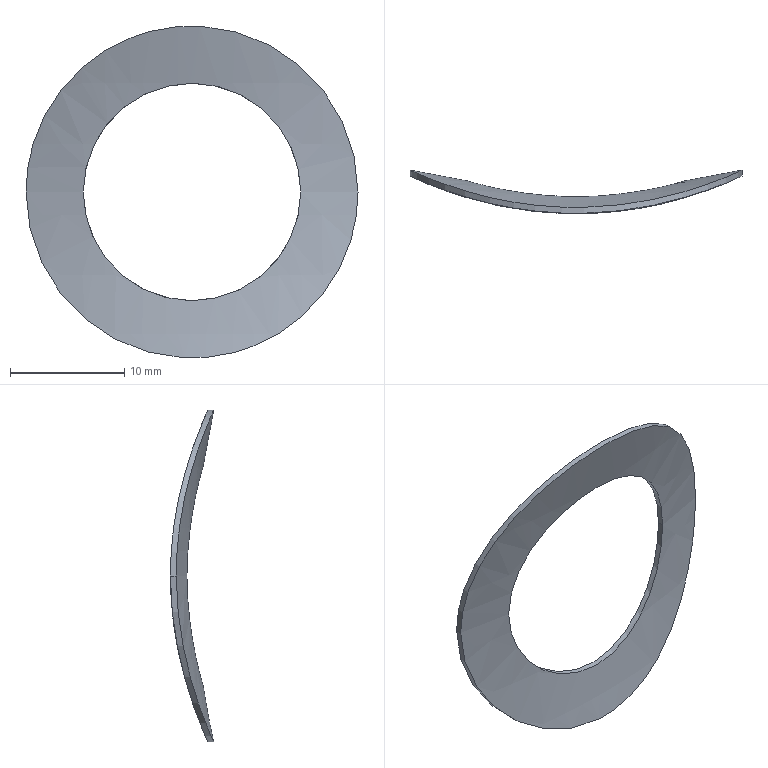Part | NX | features BREP 1 | 1 solid | 6 faces | box 29 x 3.789 x 29 mm | volume 191.933 mm3 | cylinder 4 | torus 2 | commonest cylinder face diameters 19 x2 29 x2
STEP:
#1=CARTESIAN_POINT('',(-264.193,-157.362,-153.339));
#2=VERTEX_POINT('',#1);
#3=CARTESIAN_POINT('',(-293.193,-157.362,-153.339));
#4=VERTEX_POINT('',#3);
#5=CARTESIAN_POINT('',(-264.193,-157.362,-153.339));
#6=CARTESIAN_POINT('',(-264.193,-157.362,-149.457));
#7=CARTESIAN_POINT('',(-266.594,-158.58,-143.888));
#8=CARTESIAN_POINT('',(-272.929,-160.276,-139.628));
#9=CARTESIAN_POINT('',(-278.667,-160.818,-138.448));
#10=CARTESIAN_POINT('',(-284.442,-160.279,-139.615));
#11=CARTESIAN_POINT('',(-289.203,-159.013,-142.828));
#12=CARTESIAN_POINT('',(-292.404,-157.737,-147.574));
#13=CARTESIAN_POINT('',(-293.193,-157.362,-151.397));
#14=CARTESIAN_POINT('',(-293.193,-157.362,-153.339));
#15=B_SPLINE_CURVE_WITH_KNOTS('',3,(#5,#6,#7,#8,#9,#10,#11,#12,#13,#14),.UNSPECIFIED.,.F.,.F.,(4,1,1,1,1,1,1,4),(0.,0.01147,0.0172,0.02294,0.02867,0.03441,0.04014,0.04588),.UNSPECIFIED.);
#16=EDGE_CURVE('',#2,#4,#15,.T.);
#17=ORIENTED_EDGE('',*,*,#16,.F.);
#18=CARTESIAN_POINT('',(-293.193,-157.362,-153.339));
#19=CARTESIAN_POINT('',(-293.193,-157.362,-157.221));
#20=CARTESIAN_POINT('',(-290.792,-158.58,-162.79));
#21=CARTESIAN_POINT('',(-284.457,-160.276,-167.05));
#22=CARTESIAN_POINT('',(-278.719,-160.818,-168.23));
#23=CARTESIAN_POINT('',(-272.944,-160.279,-167.063));
#24=CARTESIAN_POINT('',(-268.183,-159.013,-163.85));
#25=CARTESIAN_POINT('',(-264.982,-157.737,-159.104));
#26=CARTESIAN_POINT('',(-264.193,-157.362,-155.281));
#27=CARTESIAN_POINT('',(-264.193,-157.362,-153.339));
#28=B_SPLINE_CURVE_WITH_KNOTS('',3,(#18,#19,#20,#21,#22,#23,#24,#25,#26,#27),.UNSPECIFIED.,.F.,.F.,(4,1,1,1,1,1,1,4),(0.,0.01147,0.0172,0.02294,0.02867,0.03441,0.04014,0.04588),.UNSPECIFIED.);
#29=EDGE_CURVE('',#4,#2,#28,.T.);
#30=ORIENTED_EDGE('',*,*,#29,.F.);
#31=EDGE_LOOP('',(#17,#30));
#32=FACE_BOUND('',#31,.T.);
#33=CARTESIAN_POINT('',(-269.193,-158.302,-153.339));
#34=VERTEX_POINT('',#33);
#35=CARTESIAN_POINT('',(-288.193,-158.302,-153.339));
#36=VERTEX_POINT('',#35);
#37=CARTESIAN_POINT('',(-269.193,-158.302,-153.339));
#38=CARTESIAN_POINT('',(-269.193,-158.302,-150.815));
#39=CARTESIAN_POINT('',(-271.253,-159.004,-145.916));
#40=CARTESIAN_POINT('',(-278.678,-160.045,-142.802));
#41=CARTESIAN_POINT('',(-286.137,-159.005,-145.911));
#42=CARTESIAN_POINT('',(-288.193,-158.302,-150.815));
#43=CARTESIAN_POINT('',(-288.193,-158.302,-153.339));
#44=B_SPLINE_CURVE_WITH_KNOTS('',3,(#37,#38,#39,#40,#41,#42,#43),.UNSPECIFIED.,.F.,.F.,(4,1,1,1,4),(0.,0.007462,0.01492,0.02239,0.02985),.UNSPECIFIED.);
#45=EDGE_CURVE('',#34,#36,#44,.T.);
#46=ORIENTED_EDGE('',*,*,#45,.T.);
#47=CARTESIAN_POINT('',(-288.193,-158.302,-153.339));
#48=CARTESIAN_POINT('',(-288.193,-158.302,-155.863));
#49=CARTESIAN_POINT('',(-286.133,-159.004,-160.762));
#50=CARTESIAN_POINT('',(-278.708,-160.045,-163.876));
#51=CARTESIAN_POINT('',(-271.249,-159.005,-160.767));
#52=CARTESIAN_POINT('',(-269.193,-158.302,-155.863));
#53=CARTESIAN_POINT('',(-269.193,-158.302,-153.339));
#54=B_SPLINE_CURVE_WITH_KNOTS('',3,(#47,#48,#49,#50,#51,#52,#53),.UNSPECIFIED.,.F.,.F.,(4,1,1,1,4),(0.,0.007462,0.01492,0.02239,0.02985),.UNSPECIFIED.);
#55=EDGE_CURVE('',#36,#34,#54,.T.);
#56=ORIENTED_EDGE('',*,*,#55,.T.);
#57=EDGE_LOOP('',(#46,#56));
#58=FACE_BOUND('',#57,.T.);
#59=CARTESIAN_POINT('',(-278.693,-94.,-153.339));
#60=DIRECTION('',(0.,0.,1.));
#61=DIRECTION('',(0.2246,0.9745,0.));
#62=AXIS2_PLACEMENT_3D('',#59,#60,#61);
#63=TOROIDAL_SURFACE('',#62,130.,65.);
#64=ADVANCED_FACE('',(#32,#58),#63,.T.);
#65=CARTESIAN_POINT('',(-264.193,-157.875,-153.339));
#66=VERTEX_POINT('',#65);
#67=CARTESIAN_POINT('',(-264.193,-157.875,-153.339));
#68=DIRECTION('',(0.,1.,0.));
#69=VECTOR('',#68,1000.);
#70=LINE('',#67,#69);
#71=EDGE_CURVE('',#2,#66,#70,.F.);
#72=ORIENTED_EDGE('',*,*,#71,.F.);
#73=ORIENTED_EDGE('',*,*,#16,.T.);
#74=CARTESIAN_POINT('',(-293.193,-157.875,-153.339));
#75=VERTEX_POINT('',#74);
#76=CARTESIAN_POINT('',(-293.193,-157.875,-153.339));
#77=DIRECTION('',(0.,1.,0.));
#78=VECTOR('',#77,1000.);
#79=LINE('',#76,#78);
#80=EDGE_CURVE('',#4,#75,#79,.F.);
#81=ORIENTED_EDGE('',*,*,#80,.T.);
#82=CARTESIAN_POINT('',(-264.193,-157.875,-153.339));
#83=CARTESIAN_POINT('',(-264.193,-157.875,-149.457));
#84=CARTESIAN_POINT('',(-266.594,-159.092,-143.888));
#85=CARTESIAN_POINT('',(-272.929,-160.789,-139.628));
#86=CARTESIAN_POINT('',(-278.667,-161.331,-138.448));
#87=CARTESIAN_POINT('',(-284.442,-160.792,-139.615));
#88=CARTESIAN_POINT('',(-289.203,-159.525,-142.827));
#89=CARTESIAN_POINT('',(-292.404,-158.25,-147.574));
#90=CARTESIAN_POINT('',(-293.193,-157.875,-151.397));
#91=CARTESIAN_POINT('',(-293.193,-157.875,-153.339));
#92=B_SPLINE_CURVE_WITH_KNOTS('',3,(#82,#83,#84,#85,#86,#87,#88,#89,#90,#91),.UNSPECIFIED.,.F.,.F.,(4,1,1,1,1,1,1,4),(0.,0.01147,0.0172,0.02294,0.02867,0.03441,0.04014,0.04588),.UNSPECIFIED.);
#93=EDGE_CURVE('',#66,#75,#92,.T.);
#94=ORIENTED_EDGE('',*,*,#93,.F.);
#95=EDGE_LOOP('',(#72,#73,#81,#94));
#96=FACE_BOUND('',#95,.T.);
#97=CARTESIAN_POINT('',(-278.693,-157.319,-153.339));
#98=DIRECTION('',(0.,-1.,0.));
#99=DIRECTION('',(-1.,0.,0.));
#100=AXIS2_PLACEMENT_3D('',#97,#98,#99);
#101=CYLINDRICAL_SURFACE('',#100,14.5);
#102=ADVANCED_FACE('',(#96),#101,.T.);
#103=ORIENTED_EDGE('',*,*,#71,.T.);
#104=CARTESIAN_POINT('',(-293.193,-157.875,-153.339));
#105=CARTESIAN_POINT('',(-293.193,-157.875,-157.221));
#106=CARTESIAN_POINT('',(-290.792,-159.092,-162.79));
#107=CARTESIAN_POINT('',(-284.457,-160.789,-167.05));
#108=CARTESIAN_POINT('',(-278.719,-161.331,-168.23));
#109=CARTESIAN_POINT('',(-272.944,-160.792,-167.063));
#110=CARTESIAN_POINT('',(-268.183,-159.525,-163.851));
#111=CARTESIAN_POINT('',(-264.982,-158.25,-159.104));
#112=CARTESIAN_POINT('',(-264.193,-157.875,-155.281));
#113=CARTESIAN_POINT('',(-264.193,-157.875,-153.339));
#114=B_SPLINE_CURVE_WITH_KNOTS('',3,(#104,#105,#106,#107,#108,#109,#110,#111,#112,#113),.UNSPECIFIED.,.F.,.F.,(4,1,1,1,1,1,1,4),(0.,0.01147,0.0172,0.02294,0.02867,0.03441,0.04014,0.04588),.UNSPECIFIED.);
#115=EDGE_CURVE('',#75,#66,#114,.T.);
#116=ORIENTED_EDGE('',*,*,#115,.F.);
#117=ORIENTED_EDGE('',*,*,#80,.F.);
#118=ORIENTED_EDGE('',*,*,#29,.T.);
#119=EDGE_LOOP('',(#103,#116,#117,#118));
#120=FACE_BOUND('',#119,.T.);
#121=CARTESIAN_POINT('',(-278.693,-157.319,-153.339));
#122=DIRECTION('',(0.,-1.,0.));
#123=DIRECTION('',(-1.,0.,0.));
#124=AXIS2_PLACEMENT_3D('',#121,#122,#123);
#125=CYLINDRICAL_SURFACE('',#124,14.5);
#126=ADVANCED_FACE('',(#120),#125,.T.);
#127=CARTESIAN_POINT('',(-269.193,-158.807,-153.339));
#128=VERTEX_POINT('',#127);
#129=CARTESIAN_POINT('',(-269.193,-158.807,-153.339));
#130=DIRECTION('',(0.,1.,0.));
#131=VECTOR('',#130,1000.);
#132=LINE('',#129,#131);
#133=EDGE_CURVE('',#34,#128,#132,.F.);
#134=ORIENTED_EDGE('',*,*,#133,.F.);
#135=ORIENTED_EDGE('',*,*,#55,.F.);
#136=CARTESIAN_POINT('',(-288.193,-158.807,-153.339));
#137=VERTEX_POINT('',#136);
#138=CARTESIAN_POINT('',(-288.193,-158.807,-153.339));
#139=DIRECTION('',(0.,1.,0.));
#140=VECTOR('',#139,1000.);
#141=LINE('',#138,#140);
#142=EDGE_CURVE('',#36,#137,#141,.F.);
#143=ORIENTED_EDGE('',*,*,#142,.T.);
#144=CARTESIAN_POINT('',(-269.193,-158.807,-153.339));
#145=CARTESIAN_POINT('',(-269.193,-158.807,-155.863));
#146=CARTESIAN_POINT('',(-271.253,-159.509,-160.762));
#147=CARTESIAN_POINT('',(-278.678,-160.55,-163.876));
#148=CARTESIAN_POINT('',(-286.137,-159.51,-160.767));
#149=CARTESIAN_POINT('',(-288.193,-158.807,-155.863));
#150=CARTESIAN_POINT('',(-288.193,-158.807,-153.339));
#151=B_SPLINE_CURVE_WITH_KNOTS('',3,(#144,#145,#146,#147,#148,#149,#150),.UNSPECIFIED.,.F.,.F.,(4,1,1,1,4),(0.,0.007462,0.01492,0.02239,0.02985),.UNSPECIFIED.);
#152=EDGE_CURVE('',#128,#137,#151,.T.);
#153=ORIENTED_EDGE('',*,*,#152,.F.);
#154=EDGE_LOOP('',(#134,#135,#143,#153));
#155=FACE_BOUND('',#154,.T.);
#156=CARTESIAN_POINT('',(-278.693,-158.289,-153.339));
#157=DIRECTION('',(0.,-1.,0.));
#158=DIRECTION('',(-1.,0.,0.));
#159=AXIS2_PLACEMENT_3D('',#156,#157,#158);
#160=CYLINDRICAL_SURFACE('',#159,9.5);
#161=ADVANCED_FACE('',(#155),#160,.F.);
#162=ORIENTED_EDGE('',*,*,#133,.T.);
#163=CARTESIAN_POINT('',(-288.193,-158.807,-153.339));
#164=CARTESIAN_POINT('',(-288.193,-158.807,-150.815));
#165=CARTESIAN_POINT('',(-286.133,-159.509,-145.916));
#166=CARTESIAN_POINT('',(-278.708,-160.55,-142.802));
#167=CARTESIAN_POINT('',(-271.249,-159.51,-145.911));
#168=CARTESIAN_POINT('',(-269.193,-158.807,-150.815));
#169=CARTESIAN_POINT('',(-269.193,-158.807,-153.339));
#170=B_SPLINE_CURVE_WITH_KNOTS('',3,(#163,#164,#165,#166,#167,#168,#169),.UNSPECIFIED.,.F.,.F.,(4,1,1,1,4),(0.,0.007462,0.01492,0.02239,0.02985),.UNSPECIFIED.);
#171=EDGE_CURVE('',#137,#128,#170,.T.);
#172=ORIENTED_EDGE('',*,*,#171,.F.);
#173=ORIENTED_EDGE('',*,*,#142,.F.);
#174=ORIENTED_EDGE('',*,*,#45,.F.);
#175=EDGE_LOOP('',(#162,#172,#173,#174));
#176=FACE_BOUND('',#175,.T.);
#177=CARTESIAN_POINT('',(-278.693,-158.289,-153.339));
#178=DIRECTION('',(0.,-1.,0.));
#179=DIRECTION('',(-1.,0.,0.));
#180=AXIS2_PLACEMENT_3D('',#177,#178,#179);
#181=CYLINDRICAL_SURFACE('',#180,9.5);
#182=ADVANCED_FACE('',(#176),#181,.F.);
#183=ORIENTED_EDGE('',*,*,#115,.T.);
#184=ORIENTED_EDGE('',*,*,#93,.T.);
#185=EDGE_LOOP('',(#183,#184));
#186=FACE_BOUND('',#185,.T.);
#187=ORIENTED_EDGE('',*,*,#171,.T.);
#188=ORIENTED_EDGE('',*,*,#152,.T.);
#189=EDGE_LOOP('',(#187,#188));
#190=FACE_BOUND('',#189,.T.);
#191=CARTESIAN_POINT('',(-278.693,-94.,-153.339));
#192=DIRECTION('',(0.,0.,1.));
#193=DIRECTION('',(0.2229,0.9748,0.));
#194=AXIS2_PLACEMENT_3D('',#191,#192,#193);
#195=TOROIDAL_SURFACE('',#194,130.,64.5);
#196=ADVANCED_FACE('',(#186,#190),#195,.F.);
#197=CLOSED_SHELL('',(#64,#102,#126,#161,#182,#196));
#198=MANIFOLD_SOLID_BREP('',#197);
#199=(LENGTH_UNIT()NAMED_UNIT(*)SI_UNIT(.MILLI.,.METRE.));
#200=UNCERTAINTY_MEASURE_WITH_UNIT(LENGTH_MEASURE(0.0508),#199,'','');
#201=(NAMED_UNIT(*)PLANE_ANGLE_UNIT()SI_UNIT($,.RADIAN.));
#202=(NAMED_UNIT(*)SI_UNIT($,.STERADIAN.)SOLID_ANGLE_UNIT());
#203=(GEOMETRIC_REPRESENTATION_CONTEXT(3)GLOBAL_UNCERTAINTY_ASSIGNED_CONTEXT((#200))GLOBAL_UNIT_ASSIGNED_CONTEXT((#199,#201,#202))REPRESENTATION_CONTEXT('',''));
#204=ADVANCED_BREP_SHAPE_REPRESENTATION('',(#198),#203);